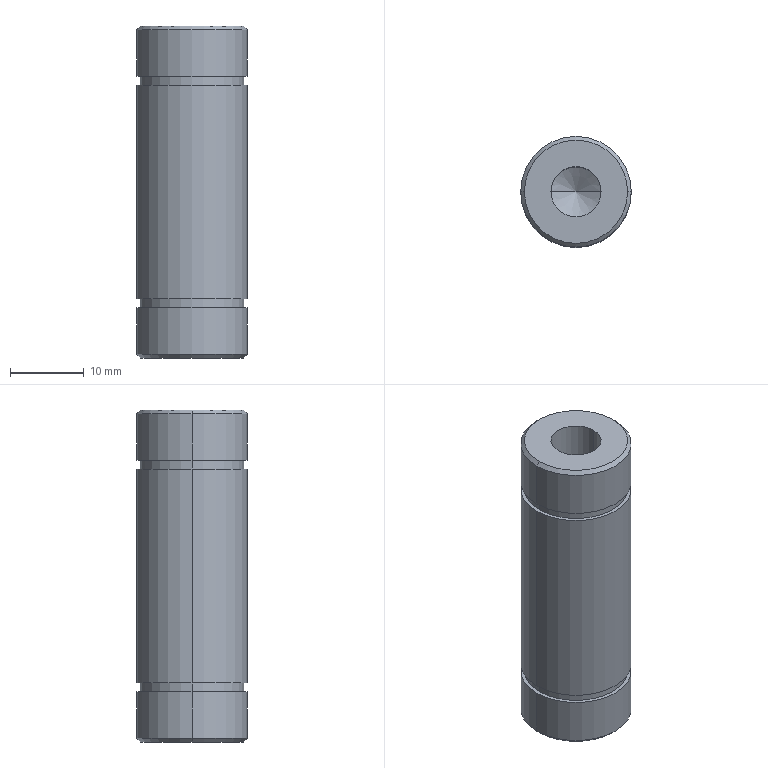Part | SolidWorks | features MirrorPattern 2, Chamfer 1, Extrusion 1, HoleWzd 1, RevCut 1 | 1 solid | 28 faces | box 15 x 15 x 45 mm | volume 6384 mm3 | cylinder 14 | cone 8 | plane 6 | commonest cylinder face diameters 15 x6 6.8 x4 14 x4
STEP:
#1=CARTESIAN_POINT('',(-7.5,0.,22.));
#2=VERTEX_POINT('',#1);
#3=CARTESIAN_POINT('',(7.5,0.,22.));
#4=VERTEX_POINT('',#3);
#5=CARTESIAN_POINT('',(0.,0.,22.));
#6=DIRECTION('',(0.,0.,-1.));
#7=DIRECTION('',(1.,0.,0.));
#8=AXIS2_PLACEMENT_3D('',#5,#6,#7);
#9=CIRCLE('',#8,7.5);
#10=EDGE_CURVE('',#2,#4,#9,.T.);
#11=ORIENTED_EDGE('',*,*,#10,.T.);
#12=CARTESIAN_POINT('',(7.5,0.,15.7));
#13=VERTEX_POINT('',#12);
#14=CARTESIAN_POINT('',(7.5,0.,22.5));
#15=DIRECTION('',(0.,0.,-1.));
#16=VECTOR('',#15,1000.);
#17=LINE('',#14,#16);
#18=EDGE_CURVE('',#4,#13,#17,.T.);
#19=ORIENTED_EDGE('',*,*,#18,.T.);
#20=CARTESIAN_POINT('',(-7.5,0.,15.7));
#21=VERTEX_POINT('',#20);
#22=CARTESIAN_POINT('',(0.,0.,15.7));
#23=DIRECTION('',(0.,0.,-1.));
#24=DIRECTION('',(-1.,0.,0.));
#25=AXIS2_PLACEMENT_3D('',#22,#23,#24);
#26=CIRCLE('',#25,7.5);
#27=EDGE_CURVE('',#21,#13,#26,.T.);
#28=ORIENTED_EDGE('',*,*,#27,.F.);
#29=CARTESIAN_POINT('',(-7.5,0.,22.5));
#30=DIRECTION('',(0.,0.,-1.));
#31=VECTOR('',#30,1000.);
#32=LINE('',#29,#31);
#33=EDGE_CURVE('',#2,#21,#32,.T.);
#34=ORIENTED_EDGE('',*,*,#33,.F.);
#35=EDGE_LOOP('',(#11,#19,#28,#34));
#36=FACE_OUTER_BOUND('',#35,.T.);
#37=CARTESIAN_POINT('',(0.,0.,22.5));
#38=DIRECTION('',(0.,0.,-1.));
#39=DIRECTION('',(-1.,0.,0.));
#40=AXIS2_PLACEMENT_3D('',#37,#38,#39);
#41=CYLINDRICAL_SURFACE('',#40,7.5);
#42=ADVANCED_FACE('',(#36),#41,.T.);
#43=CARTESIAN_POINT('',(7.,0.,22.5));
#44=VERTEX_POINT('',#43);
#45=CARTESIAN_POINT('',(-7.,0.,22.5));
#46=VERTEX_POINT('',#45);
#47=CARTESIAN_POINT('',(0.,0.,22.5));
#48=DIRECTION('',(0.,0.,1.));
#49=DIRECTION('',(1.,0.,0.));
#50=AXIS2_PLACEMENT_3D('',#47,#48,#49);
#51=CIRCLE('',#50,7.);
#52=EDGE_CURVE('',#44,#46,#51,.T.);
#53=ORIENTED_EDGE('',*,*,#52,.F.);
#54=CARTESIAN_POINT('',(7.,0.,22.5));
#55=DIRECTION('',(0.7071,0.,-0.7071));
#56=VECTOR('',#55,1000.);
#57=LINE('',#54,#56);
#58=EDGE_CURVE('',#44,#4,#57,.T.);
#59=ORIENTED_EDGE('',*,*,#58,.T.);
#60=ORIENTED_EDGE('',*,*,#10,.F.);
#61=CARTESIAN_POINT('',(-7.,0.,22.5));
#62=DIRECTION('',(-0.7071,0.,-0.7071));
#63=VECTOR('',#62,1000.);
#64=LINE('',#61,#63);
#65=EDGE_CURVE('',#46,#2,#64,.T.);
#66=ORIENTED_EDGE('',*,*,#65,.F.);
#67=EDGE_LOOP('',(#53,#59,#60,#66));
#68=FACE_OUTER_BOUND('',#67,.T.);
#69=CARTESIAN_POINT('',(0.,0.,22.5));
#70=DIRECTION('',(0.,0.,-1.));
#71=DIRECTION('',(-1.,0.,0.));
#72=AXIS2_PLACEMENT_3D('',#69,#70,#71);
#73=CONICAL_SURFACE('',#72,7.,0.7854);
#74=ADVANCED_FACE('',(#68),#73,.T.);
#75=CARTESIAN_POINT('',(-3.4,0.,2.5));
#76=VERTEX_POINT('',#75);
#77=CARTESIAN_POINT('',(3.4,0.,2.5));
#78=VERTEX_POINT('',#77);
#79=CARTESIAN_POINT('',(0.,0.,2.5));
#80=DIRECTION('',(0.,0.,1.));
#81=DIRECTION('',(1.,0.,0.));
#82=AXIS2_PLACEMENT_3D('',#79,#80,#81);
#83=CIRCLE('',#82,3.4);
#84=EDGE_CURVE('',#76,#78,#83,.T.);
#85=ORIENTED_EDGE('',*,*,#84,.F.);
#86=CARTESIAN_POINT('',(-3.4,0.,22.5));
#87=VERTEX_POINT('',#86);
#88=CARTESIAN_POINT('',(-3.4,0.,22.5));
#89=DIRECTION('',(0.,0.,1.));
#90=VECTOR('',#89,1000.);
#91=LINE('',#88,#90);
#92=EDGE_CURVE('',#76,#87,#91,.T.);
#93=ORIENTED_EDGE('',*,*,#92,.T.);
#94=CARTESIAN_POINT('',(3.4,0.,22.5));
#95=VERTEX_POINT('',#94);
#96=CARTESIAN_POINT('',(0.,0.,22.5));
#97=DIRECTION('',(0.,0.,1.));
#98=DIRECTION('',(1.,0.,0.));
#99=AXIS2_PLACEMENT_3D('',#96,#97,#98);
#100=CIRCLE('',#99,3.4);
#101=EDGE_CURVE('',#87,#95,#100,.T.);
#102=ORIENTED_EDGE('',*,*,#101,.T.);
#103=CARTESIAN_POINT('',(3.4,0.,22.5));
#104=DIRECTION('',(0.,0.,1.));
#105=VECTOR('',#104,1000.);
#106=LINE('',#103,#105);
#107=EDGE_CURVE('',#78,#95,#106,.T.);
#108=ORIENTED_EDGE('',*,*,#107,.F.);
#109=EDGE_LOOP('',(#85,#93,#102,#108));
#110=FACE_OUTER_BOUND('',#109,.T.);
#111=CARTESIAN_POINT('',(0.,0.,22.5));
#112=DIRECTION('',(0.,0.,1.));
#113=DIRECTION('',(1.,0.,0.));
#114=AXIS2_PLACEMENT_3D('',#111,#112,#113);
#115=CYLINDRICAL_SURFACE('',#114,3.4);
#116=ADVANCED_FACE('',(#110),#115,.F.);
#117=CARTESIAN_POINT('',(0.,0.,0.4571));
#118=VERTEX_POINT('',#117);
#119=CARTESIAN_POINT('',(3.4,0.,2.5));
#120=DIRECTION('',(0.8572,0.,0.515));
#121=VECTOR('',#120,1000.);
#122=LINE('',#119,#121);
#123=EDGE_CURVE('',#118,#78,#122,.T.);
#124=ORIENTED_EDGE('',*,*,#123,.F.);
#125=CARTESIAN_POINT('',(-3.4,0.,2.5));
#126=DIRECTION('',(-0.8572,0.,0.515));
#127=VECTOR('',#126,1000.);
#128=LINE('',#125,#127);
#129=EDGE_CURVE('',#118,#76,#128,.T.);
#130=ORIENTED_EDGE('',*,*,#129,.T.);
#131=ORIENTED_EDGE('',*,*,#84,.T.);
#132=EDGE_LOOP('',(#124,#130,#131));
#133=FACE_OUTER_BOUND('',#132,.T.);
#134=CARTESIAN_POINT('',(0.,0.,2.5));
#135=DIRECTION('',(0.,0.,1.));
#136=DIRECTION('',(1.,0.,0.));
#137=AXIS2_PLACEMENT_3D('',#134,#135,#136);
#138=CONICAL_SURFACE('',#137,3.4,1.03);
#139=ADVANCED_FACE('',(#133),#138,.F.);
#140=CARTESIAN_POINT('',(7.,0.,14.5));
#141=VERTEX_POINT('',#140);
#142=CARTESIAN_POINT('',(-7.,0.,14.5));
#143=VERTEX_POINT('',#142);
#144=CARTESIAN_POINT('',(0.,0.,14.5));
#145=DIRECTION('',(0.,0.,-1.));
#146=DIRECTION('',(-1.,0.,0.));
#147=AXIS2_PLACEMENT_3D('',#144,#145,#146);
#148=CIRCLE('',#147,7.);
#149=EDGE_CURVE('',#141,#143,#148,.T.);
#150=ORIENTED_EDGE('',*,*,#149,.F.);
#151=CARTESIAN_POINT('',(7.,0.,15.7));
#152=VERTEX_POINT('',#151);
#153=CARTESIAN_POINT('',(7.,0.,24.689));
#154=DIRECTION('',(0.,0.,1.));
#155=VECTOR('',#154,1000.);
#156=LINE('',#153,#155);
#157=EDGE_CURVE('',#141,#152,#156,.T.);
#158=ORIENTED_EDGE('',*,*,#157,.T.);
#159=CARTESIAN_POINT('',(-7.,0.,15.7));
#160=VERTEX_POINT('',#159);
#161=CARTESIAN_POINT('',(0.,0.,15.7));
#162=DIRECTION('',(0.,0.,-1.));
#163=DIRECTION('',(-1.,0.,0.));
#164=AXIS2_PLACEMENT_3D('',#161,#162,#163);
#165=CIRCLE('',#164,7.);
#166=EDGE_CURVE('',#152,#160,#165,.T.);
#167=ORIENTED_EDGE('',*,*,#166,.T.);
#168=CARTESIAN_POINT('',(-7.,0.,24.689));
#169=DIRECTION('',(0.,0.,1.));
#170=VECTOR('',#169,1000.);
#171=LINE('',#168,#170);
#172=EDGE_CURVE('',#143,#160,#171,.T.);
#173=ORIENTED_EDGE('',*,*,#172,.F.);
#174=EDGE_LOOP('',(#150,#158,#167,#173));
#175=FACE_OUTER_BOUND('',#174,.T.);
#176=CARTESIAN_POINT('',(0.,0.,24.689));
#177=DIRECTION('',(0.,0.,1.));
#178=DIRECTION('',(-1.,0.,0.));
#179=AXIS2_PLACEMENT_3D('',#176,#177,#178);
#180=CYLINDRICAL_SURFACE('',#179,7.);
#181=ADVANCED_FACE('',(#175),#180,.T.);
#182=CARTESIAN_POINT('',(-7.5,0.,-15.7));
#183=VERTEX_POINT('',#182);
#184=CARTESIAN_POINT('',(7.5,0.,-15.7));
#185=VERTEX_POINT('',#184);
#186=CARTESIAN_POINT('',(0.,0.,-15.7));
#187=DIRECTION('',(0.,0.,-1.));
#188=DIRECTION('',(-1.,0.,0.));
#189=AXIS2_PLACEMENT_3D('',#186,#187,#188);
#190=CIRCLE('',#189,7.5);
#191=EDGE_CURVE('',#183,#185,#190,.T.);
#192=ORIENTED_EDGE('',*,*,#191,.T.);
#193=CARTESIAN_POINT('',(7.5,0.,-22.));
#194=VERTEX_POINT('',#193);
#195=CARTESIAN_POINT('',(7.5,0.,22.5));
#196=DIRECTION('',(0.,0.,-1.));
#197=VECTOR('',#196,1000.);
#198=LINE('',#195,#197);
#199=EDGE_CURVE('',#185,#194,#198,.T.);
#200=ORIENTED_EDGE('',*,*,#199,.T.);
#201=CARTESIAN_POINT('',(-7.5,0.,-22.));
#202=VERTEX_POINT('',#201);
#203=CARTESIAN_POINT('',(0.,0.,-22.));
#204=DIRECTION('',(0.,0.,1.));
#205=DIRECTION('',(1.,0.,0.));
#206=AXIS2_PLACEMENT_3D('',#203,#204,#205);
#207=CIRCLE('',#206,7.5);
#208=EDGE_CURVE('',#194,#202,#207,.T.);
#209=ORIENTED_EDGE('',*,*,#208,.T.);
#210=CARTESIAN_POINT('',(-7.5,0.,22.5));
#211=DIRECTION('',(0.,0.,-1.));
#212=VECTOR('',#211,1000.);
#213=LINE('',#210,#212);
#214=EDGE_CURVE('',#183,#202,#213,.T.);
#215=ORIENTED_EDGE('',*,*,#214,.F.);
#216=EDGE_LOOP('',(#192,#200,#209,#215));
#217=FACE_OUTER_BOUND('',#216,.T.);
#218=CARTESIAN_POINT('',(0.,0.,22.5));
#219=DIRECTION('',(0.,0.,-1.));
#220=DIRECTION('',(-1.,0.,0.));
#221=AXIS2_PLACEMENT_3D('',#218,#219,#220);
#222=CYLINDRICAL_SURFACE('',#221,7.5);
#223=ADVANCED_FACE('',(#217),#222,.T.);
#224=CARTESIAN_POINT('',(-7.,0.,-22.5));
#225=VERTEX_POINT('',#224);
#226=CARTESIAN_POINT('',(7.,0.,-22.5));
#227=VERTEX_POINT('',#226);
#228=CARTESIAN_POINT('',(0.,0.,-22.5));
#229=DIRECTION('',(0.,0.,-1.));
#230=DIRECTION('',(1.,0.,0.));
#231=AXIS2_PLACEMENT_3D('',#228,#229,#230);
#232=CIRCLE('',#231,7.);
#233=EDGE_CURVE('',#225,#227,#232,.T.);
#234=ORIENTED_EDGE('',*,*,#233,.F.);
#235=CARTESIAN_POINT('',(-7.5,0.,-22.));
#236=DIRECTION('',(-0.7071,0.,0.7071));
#237=VECTOR('',#236,1000.);
#238=LINE('',#235,#237);
#239=EDGE_CURVE('',#225,#202,#238,.T.);
#240=ORIENTED_EDGE('',*,*,#239,.T.);
#241=ORIENTED_EDGE('',*,*,#208,.F.);
#242=CARTESIAN_POINT('',(7.5,0.,-22.));
#243=DIRECTION('',(0.7071,0.,0.7071));
#244=VECTOR('',#243,1000.);
#245=LINE('',#242,#244);
#246=EDGE_CURVE('',#227,#194,#245,.T.);
#247=ORIENTED_EDGE('',*,*,#246,.F.);
#248=EDGE_LOOP('',(#234,#240,#241,#247));
#249=FACE_OUTER_BOUND('',#248,.T.);
#250=CARTESIAN_POINT('',(0.,0.,-22.));
#251=DIRECTION('',(0.,0.,1.));
#252=DIRECTION('',(1.,0.,0.));
#253=AXIS2_PLACEMENT_3D('',#250,#251,#252);
#254=CONICAL_SURFACE('',#253,7.5,0.7854);
#255=ADVANCED_FACE('',(#249),#254,.T.);
#256=CARTESIAN_POINT('',(3.4,0.,-2.5));
#257=VERTEX_POINT('',#256);
#258=CARTESIAN_POINT('',(-3.4,0.,-2.5));
#259=VERTEX_POINT('',#258);
#260=CARTESIAN_POINT('',(0.,0.,-2.5));
#261=DIRECTION('',(0.,0.,-1.));
#262=DIRECTION('',(-1.,0.,0.));
#263=AXIS2_PLACEMENT_3D('',#260,#261,#262);
#264=CIRCLE('',#263,3.4);
#265=EDGE_CURVE('',#257,#259,#264,.T.);
#266=ORIENTED_EDGE('',*,*,#265,.F.);
#267=CARTESIAN_POINT('',(3.4,0.,-22.5));
#268=VERTEX_POINT('',#267);
#269=CARTESIAN_POINT('',(3.4,0.,-22.5));
#270=DIRECTION('',(0.,0.,-1.));
#271=VECTOR('',#270,1000.);
#272=LINE('',#269,#271);
#273=EDGE_CURVE('',#257,#268,#272,.T.);
#274=ORIENTED_EDGE('',*,*,#273,.T.);
#275=CARTESIAN_POINT('',(-3.4,0.,-22.5));
#276=VERTEX_POINT('',#275);
#277=CARTESIAN_POINT('',(0.,0.,-22.5));
#278=DIRECTION('',(0.,0.,-1.));
#279=DIRECTION('',(-1.,0.,0.));
#280=AXIS2_PLACEMENT_3D('',#277,#278,#279);
#281=CIRCLE('',#280,3.4);
#282=EDGE_CURVE('',#268,#276,#281,.T.);
#283=ORIENTED_EDGE('',*,*,#282,.T.);
#284=CARTESIAN_POINT('',(-3.4,0.,-22.5));
#285=DIRECTION('',(0.,0.,-1.));
#286=VECTOR('',#285,1000.);
#287=LINE('',#284,#286);
#288=EDGE_CURVE('',#259,#276,#287,.T.);
#289=ORIENTED_EDGE('',*,*,#288,.F.);
#290=EDGE_LOOP('',(#266,#274,#283,#289));
#291=FACE_OUTER_BOUND('',#290,.T.);
#292=CARTESIAN_POINT('',(0.,0.,-22.5));
#293=DIRECTION('',(0.,0.,-1.));
#294=DIRECTION('',(-1.,0.,0.));
#295=AXIS2_PLACEMENT_3D('',#292,#293,#294);
#296=CYLINDRICAL_SURFACE('',#295,3.4);
#297=ADVANCED_FACE('',(#291),#296,.F.);
#298=CARTESIAN_POINT('',(0.,0.,-0.4571));
#299=VERTEX_POINT('',#298);
#300=CARTESIAN_POINT('',(-3.4,0.,-2.5));
#301=DIRECTION('',(-0.8572,0.,-0.515));
#302=VECTOR('',#301,1000.);
#303=LINE('',#300,#302);
#304=EDGE_CURVE('',#299,#259,#303,.T.);
#305=ORIENTED_EDGE('',*,*,#304,.F.);
#306=CARTESIAN_POINT('',(3.4,0.,-2.5));
#307=DIRECTION('',(0.8572,0.,-0.515));
#308=VECTOR('',#307,1000.);
#309=LINE('',#306,#308);
#310=EDGE_CURVE('',#299,#257,#309,.T.);
#311=ORIENTED_EDGE('',*,*,#310,.T.);
#312=ORIENTED_EDGE('',*,*,#265,.T.);
#313=EDGE_LOOP('',(#305,#311,#312));
#314=FACE_OUTER_BOUND('',#313,.T.);
#315=CARTESIAN_POINT('',(0.,0.,-2.5));
#316=DIRECTION('',(0.,0.,-1.));
#317=DIRECTION('',(-1.,0.,0.));
#318=AXIS2_PLACEMENT_3D('',#315,#316,#317);
#319=CONICAL_SURFACE('',#318,3.4,1.03);
#320=ADVANCED_FACE('',(#314),#319,.F.);
#321=CARTESIAN_POINT('',(-7.,0.,-14.5));
#322=VERTEX_POINT('',#321);
#323=CARTESIAN_POINT('',(7.,0.,-14.5));
#324=VERTEX_POINT('',#323);
#325=CARTESIAN_POINT('',(0.,0.,-14.5));
#326=DIRECTION('',(0.,0.,-1.));
#327=DIRECTION('',(-1.,0.,0.));
#328=AXIS2_PLACEMENT_3D('',#325,#326,#327);
#329=CIRCLE('',#328,7.);
#330=EDGE_CURVE('',#322,#324,#329,.T.);
#331=ORIENTED_EDGE('',*,*,#330,.T.);
#332=CARTESIAN_POINT('',(7.,0.,-15.7));
#333=VERTEX_POINT('',#332);
#334=CARTESIAN_POINT('',(7.,0.,-24.689));
#335=DIRECTION('',(0.,0.,-1.));
#336=VECTOR('',#335,1000.);
#337=LINE('',#334,#336);
#338=EDGE_CURVE('',#324,#333,#337,.T.);
#339=ORIENTED_EDGE('',*,*,#338,.T.);
#340=CARTESIAN_POINT('',(-7.,0.,-15.7));
#341=VERTEX_POINT('',#340);
#342=CARTESIAN_POINT('',(0.,0.,-15.7));
#343=DIRECTION('',(0.,0.,-1.));
#344=DIRECTION('',(-1.,0.,0.));
#345=AXIS2_PLACEMENT_3D('',#342,#343,#344);
#346=CIRCLE('',#345,7.);
#347=EDGE_CURVE('',#341,#333,#346,.T.);
#348=ORIENTED_EDGE('',*,*,#347,.F.);
#349=CARTESIAN_POINT('',(-7.,0.,-24.689));
#350=DIRECTION('',(0.,0.,-1.));
#351=VECTOR('',#350,1000.);
#352=LINE('',#349,#351);
#353=EDGE_CURVE('',#322,#341,#352,.T.);
#354=ORIENTED_EDGE('',*,*,#353,.F.);
#355=EDGE_LOOP('',(#331,#339,#348,#354));
#356=FACE_OUTER_BOUND('',#355,.T.);
#357=CARTESIAN_POINT('',(0.,0.,-24.689));
#358=DIRECTION('',(0.,0.,-1.));
#359=DIRECTION('',(-1.,0.,0.));
#360=AXIS2_PLACEMENT_3D('',#357,#358,#359);
#361=CYLINDRICAL_SURFACE('',#360,7.);
#362=ADVANCED_FACE('',(#356),#361,.T.);
#363=CARTESIAN_POINT('',(-7.5,0.,14.5));
#364=VERTEX_POINT('',#363);
#365=CARTESIAN_POINT('',(7.5,0.,14.5));
#366=VERTEX_POINT('',#365);
#367=CARTESIAN_POINT('',(0.,0.,14.5));
#368=DIRECTION('',(0.,0.,-1.));
#369=DIRECTION('',(-1.,0.,0.));
#370=AXIS2_PLACEMENT_3D('',#367,#368,#369);
#371=CIRCLE('',#370,7.5);
#372=EDGE_CURVE('',#364,#366,#371,.T.);
#373=ORIENTED_EDGE('',*,*,#372,.T.);
#374=CARTESIAN_POINT('',(7.5,0.,-14.5));
#375=VERTEX_POINT('',#374);
#376=CARTESIAN_POINT('',(7.5,0.,22.5));
#377=DIRECTION('',(0.,0.,-1.));
#378=VECTOR('',#377,1000.);
#379=LINE('',#376,#378);
#380=EDGE_CURVE('',#366,#375,#379,.T.);
#381=ORIENTED_EDGE('',*,*,#380,.T.);
#382=CARTESIAN_POINT('',(-7.5,0.,-14.5));
#383=VERTEX_POINT('',#382);
#384=CARTESIAN_POINT('',(0.,0.,-14.5));
#385=DIRECTION('',(0.,0.,-1.));
#386=DIRECTION('',(-1.,0.,0.));
#387=AXIS2_PLACEMENT_3D('',#384,#385,#386);
#388=CIRCLE('',#387,7.5);
#389=EDGE_CURVE('',#383,#375,#388,.T.);
#390=ORIENTED_EDGE('',*,*,#389,.F.);
#391=CARTESIAN_POINT('',(-7.5,0.,22.5));
#392=DIRECTION('',(0.,0.,-1.));
#393=VECTOR('',#392,1000.);
#394=LINE('',#391,#393);
#395=EDGE_CURVE('',#364,#383,#394,.T.);
#396=ORIENTED_EDGE('',*,*,#395,.F.);
#397=EDGE_LOOP('',(#373,#381,#390,#396));
#398=FACE_OUTER_BOUND('',#397,.T.);
#399=CARTESIAN_POINT('',(0.,0.,22.5));
#400=DIRECTION('',(0.,0.,-1.));
#401=DIRECTION('',(-1.,0.,0.));
#402=AXIS2_PLACEMENT_3D('',#399,#400,#401);
#403=CYLINDRICAL_SURFACE('',#402,7.5);
#404=ADVANCED_FACE('',(#398),#403,.T.);
#405=ORIENTED_EDGE('',*,*,#380,.F.);
#406=CARTESIAN_POINT('',(0.,0.,14.5));
#407=DIRECTION('',(0.,0.,-1.));
#408=DIRECTION('',(-1.,0.,0.));
#409=AXIS2_PLACEMENT_3D('',#406,#407,#408);
#410=CIRCLE('',#409,7.5);
#411=EDGE_CURVE('',#366,#364,#410,.T.);
#412=ORIENTED_EDGE('',*,*,#411,.T.);
#413=ORIENTED_EDGE('',*,*,#395,.T.);
#414=CARTESIAN_POINT('',(0.,0.,-14.5));
#415=DIRECTION('',(0.,0.,-1.));
#416=DIRECTION('',(-1.,0.,0.));
#417=AXIS2_PLACEMENT_3D('',#414,#415,#416);
#418=CIRCLE('',#417,7.5);
#419=EDGE_CURVE('',#375,#383,#418,.T.);
#420=ORIENTED_EDGE('',*,*,#419,.F.);
#421=EDGE_LOOP('',(#405,#412,#413,#420));
#422=FACE_OUTER_BOUND('',#421,.T.);
#423=CARTESIAN_POINT('',(0.,0.,22.5));
#424=DIRECTION('',(0.,0.,-1.));
#425=DIRECTION('',(-1.,0.,0.));
#426=AXIS2_PLACEMENT_3D('',#423,#424,#425);
#427=CYLINDRICAL_SURFACE('',#426,7.5);
#428=ADVANCED_FACE('',(#422),#427,.T.);
#429=ORIENTED_EDGE('',*,*,#389,.T.);
#430=ORIENTED_EDGE('',*,*,#419,.T.);
#431=EDGE_LOOP('',(#429,#430));
#432=FACE_OUTER_BOUND('',#431,.T.);
#433=ORIENTED_EDGE('',*,*,#330,.F.);
#434=CARTESIAN_POINT('',(0.,0.,-14.5));
#435=DIRECTION('',(0.,0.,-1.));
#436=DIRECTION('',(-1.,0.,0.));
#437=AXIS2_PLACEMENT_3D('',#434,#435,#436);
#438=CIRCLE('',#437,7.);
#439=EDGE_CURVE('',#324,#322,#438,.T.);
#440=ORIENTED_EDGE('',*,*,#439,.F.);
#441=EDGE_LOOP('',(#433,#440));
#442=FACE_BOUND('',#441,.T.);
#443=CARTESIAN_POINT('',(7.5,0.,-14.5));
#444=DIRECTION('',(0.,0.,-1.));
#445=DIRECTION('',(-1.,0.,0.));
#446=AXIS2_PLACEMENT_3D('',#443,#444,#445);
#447=PLANE('',#446);
#448=ADVANCED_FACE('',(#432,#442),#447,.T.);
#449=ORIENTED_EDGE('',*,*,#338,.F.);
#450=ORIENTED_EDGE('',*,*,#439,.T.);
#451=ORIENTED_EDGE('',*,*,#353,.T.);
#452=CARTESIAN_POINT('',(0.,0.,-15.7));
#453=DIRECTION('',(0.,0.,-1.));
#454=DIRECTION('',(-1.,0.,0.));
#455=AXIS2_PLACEMENT_3D('',#452,#453,#454);
#456=CIRCLE('',#455,7.);
#457=EDGE_CURVE('',#333,#341,#456,.T.);
#458=ORIENTED_EDGE('',*,*,#457,.F.);
#459=EDGE_LOOP('',(#449,#450,#451,#458));
#460=FACE_OUTER_BOUND('',#459,.T.);
#461=CARTESIAN_POINT('',(0.,0.,-24.689));
#462=DIRECTION('',(0.,0.,-1.));
#463=DIRECTION('',(-1.,0.,0.));
#464=AXIS2_PLACEMENT_3D('',#461,#462,#463);
#465=CYLINDRICAL_SURFACE('',#464,7.);
#466=ADVANCED_FACE('',(#460),#465,.T.);
#467=ORIENTED_EDGE('',*,*,#347,.T.);
#468=ORIENTED_EDGE('',*,*,#457,.T.);
#469=EDGE_LOOP('',(#467,#468));
#470=FACE_BOUND('',#469,.T.);
#471=ORIENTED_EDGE('',*,*,#191,.F.);
#472=CARTESIAN_POINT('',(0.,0.,-15.7));
#473=DIRECTION('',(0.,0.,-1.));
#474=DIRECTION('',(-1.,0.,0.));
#475=AXIS2_PLACEMENT_3D('',#472,#473,#474);
#476=CIRCLE('',#475,7.5);
#477=EDGE_CURVE('',#185,#183,#476,.T.);
#478=ORIENTED_EDGE('',*,*,#477,.F.);
#479=EDGE_LOOP('',(#471,#478));
#480=FACE_OUTER_BOUND('',#479,.T.);
#481=CARTESIAN_POINT('',(7.5,0.,-15.7));
#482=DIRECTION('',(0.,0.,1.));
#483=DIRECTION('',(1.,0.,0.));
#484=AXIS2_PLACEMENT_3D('',#481,#482,#483);
#485=PLANE('',#484);
#486=ADVANCED_FACE('',(#470,#480),#485,.T.);
#487=ORIENTED_EDGE('',*,*,#310,.F.);
#488=ORIENTED_EDGE('',*,*,#304,.T.);
#489=CARTESIAN_POINT('',(0.,0.,-2.5));
#490=DIRECTION('',(0.,0.,-1.));
#491=DIRECTION('',(-1.,0.,0.));
#492=AXIS2_PLACEMENT_3D('',#489,#490,#491);
#493=CIRCLE('',#492,3.4);
#494=EDGE_CURVE('',#259,#257,#493,.T.);
#495=ORIENTED_EDGE('',*,*,#494,.T.);
#496=EDGE_LOOP('',(#487,#488,#495));
#497=FACE_OUTER_BOUND('',#496,.T.);
#498=CARTESIAN_POINT('',(0.,0.,-2.5));
#499=DIRECTION('',(0.,0.,-1.));
#500=DIRECTION('',(-1.,0.,0.));
#501=AXIS2_PLACEMENT_3D('',#498,#499,#500);
#502=CONICAL_SURFACE('',#501,3.4,1.03);
#503=ADVANCED_FACE('',(#497),#502,.F.);
#504=ORIENTED_EDGE('',*,*,#273,.F.);
#505=ORIENTED_EDGE('',*,*,#494,.F.);
#506=ORIENTED_EDGE('',*,*,#288,.T.);
#507=CARTESIAN_POINT('',(0.,0.,-22.5));
#508=DIRECTION('',(0.,0.,-1.));
#509=DIRECTION('',(-1.,0.,0.));
#510=AXIS2_PLACEMENT_3D('',#507,#508,#509);
#511=CIRCLE('',#510,3.4);
#512=EDGE_CURVE('',#276,#268,#511,.T.);
#513=ORIENTED_EDGE('',*,*,#512,.T.);
#514=EDGE_LOOP('',(#504,#505,#506,#513));
#515=FACE_OUTER_BOUND('',#514,.T.);
#516=CARTESIAN_POINT('',(0.,0.,-22.5));
#517=DIRECTION('',(0.,0.,-1.));
#518=DIRECTION('',(-1.,0.,0.));
#519=AXIS2_PLACEMENT_3D('',#516,#517,#518);
#520=CYLINDRICAL_SURFACE('',#519,3.4);
#521=ADVANCED_FACE('',(#515),#520,.F.);
#522=ORIENTED_EDGE('',*,*,#512,.F.);
#523=ORIENTED_EDGE('',*,*,#282,.F.);
#524=EDGE_LOOP('',(#522,#523));
#525=FACE_BOUND('',#524,.T.);
#526=CARTESIAN_POINT('',(0.,0.,-22.5));
#527=DIRECTION('',(0.,0.,-1.));
#528=DIRECTION('',(1.,0.,0.));
#529=AXIS2_PLACEMENT_3D('',#526,#527,#528);
#530=CIRCLE('',#529,7.);
#531=EDGE_CURVE('',#227,#225,#530,.T.);
#532=ORIENTED_EDGE('',*,*,#531,.T.);
#533=ORIENTED_EDGE('',*,*,#233,.T.);
#534=EDGE_LOOP('',(#532,#533));
#535=FACE_OUTER_BOUND('',#534,.T.);
#536=CARTESIAN_POINT('',(0.,0.,-22.5));
#537=DIRECTION('',(0.,0.,1.));
#538=DIRECTION('',(1.,0.,0.));
#539=AXIS2_PLACEMENT_3D('',#536,#537,#538);
#540=PLANE('',#539);
#541=ADVANCED_FACE('',(#525,#535),#540,.F.);
#542=ORIENTED_EDGE('',*,*,#239,.F.);
#543=ORIENTED_EDGE('',*,*,#531,.F.);
#544=ORIENTED_EDGE('',*,*,#246,.T.);
#545=CARTESIAN_POINT('',(0.,0.,-22.));
#546=DIRECTION('',(0.,0.,1.));
#547=DIRECTION('',(1.,0.,0.));
#548=AXIS2_PLACEMENT_3D('',#545,#546,#547);
#549=CIRCLE('',#548,7.5);
#550=EDGE_CURVE('',#202,#194,#549,.T.);
#551=ORIENTED_EDGE('',*,*,#550,.F.);
#552=EDGE_LOOP('',(#542,#543,#544,#551));
#553=FACE_OUTER_BOUND('',#552,.T.);
#554=CARTESIAN_POINT('',(0.,0.,-22.));
#555=DIRECTION('',(0.,0.,1.));
#556=DIRECTION('',(1.,0.,0.));
#557=AXIS2_PLACEMENT_3D('',#554,#555,#556);
#558=CONICAL_SURFACE('',#557,7.5,0.7854);
#559=ADVANCED_FACE('',(#553),#558,.T.);
#560=ORIENTED_EDGE('',*,*,#199,.F.);
#561=ORIENTED_EDGE('',*,*,#477,.T.);
#562=ORIENTED_EDGE('',*,*,#214,.T.);
#563=ORIENTED_EDGE('',*,*,#550,.T.);
#564=EDGE_LOOP('',(#560,#561,#562,#563));
#565=FACE_OUTER_BOUND('',#564,.T.);
#566=CARTESIAN_POINT('',(0.,0.,22.5));
#567=DIRECTION('',(0.,0.,-1.));
#568=DIRECTION('',(-1.,0.,0.));
#569=AXIS2_PLACEMENT_3D('',#566,#567,#568);
#570=CYLINDRICAL_SURFACE('',#569,7.5);
#571=ADVANCED_FACE('',(#565),#570,.T.);
#572=ORIENTED_EDGE('',*,*,#372,.F.);
#573=ORIENTED_EDGE('',*,*,#411,.F.);
#574=EDGE_LOOP('',(#572,#573));
#575=FACE_OUTER_BOUND('',#574,.T.);
#576=CARTESIAN_POINT('',(0.,0.,14.5));
#577=DIRECTION('',(0.,0.,-1.));
#578=DIRECTION('',(-1.,0.,0.));
#579=AXIS2_PLACEMENT_3D('',#576,#577,#578);
#580=CIRCLE('',#579,7.);
#581=EDGE_CURVE('',#143,#141,#580,.T.);
#582=ORIENTED_EDGE('',*,*,#581,.T.);
#583=ORIENTED_EDGE('',*,*,#149,.T.);
#584=EDGE_LOOP('',(#582,#583));
#585=FACE_BOUND('',#584,.T.);
#586=CARTESIAN_POINT('',(7.5,0.,14.5));
#587=DIRECTION('',(0.,0.,1.));
#588=DIRECTION('',(-1.,0.,0.));
#589=AXIS2_PLACEMENT_3D('',#586,#587,#588);
#590=PLANE('',#589);
#591=ADVANCED_FACE('',(#575,#585),#590,.T.);
#592=ORIENTED_EDGE('',*,*,#157,.F.);
#593=ORIENTED_EDGE('',*,*,#581,.F.);
#594=ORIENTED_EDGE('',*,*,#172,.T.);
#595=CARTESIAN_POINT('',(0.,0.,15.7));
#596=DIRECTION('',(0.,0.,-1.));
#597=DIRECTION('',(-1.,0.,0.));
#598=AXIS2_PLACEMENT_3D('',#595,#596,#597);
#599=CIRCLE('',#598,7.);
#600=EDGE_CURVE('',#160,#152,#599,.T.);
#601=ORIENTED_EDGE('',*,*,#600,.T.);
#602=EDGE_LOOP('',(#592,#593,#594,#601));
#603=FACE_OUTER_BOUND('',#602,.T.);
#604=CARTESIAN_POINT('',(0.,0.,24.689));
#605=DIRECTION('',(0.,0.,1.));
#606=DIRECTION('',(-1.,0.,0.));
#607=AXIS2_PLACEMENT_3D('',#604,#605,#606);
#608=CYLINDRICAL_SURFACE('',#607,7.);
#609=ADVANCED_FACE('',(#603),#608,.T.);
#610=ORIENTED_EDGE('',*,*,#600,.F.);
#611=ORIENTED_EDGE('',*,*,#166,.F.);
#612=EDGE_LOOP('',(#610,#611));
#613=FACE_BOUND('',#612,.T.);
#614=ORIENTED_EDGE('',*,*,#27,.T.);
#615=CARTESIAN_POINT('',(0.,0.,15.7));
#616=DIRECTION('',(0.,0.,-1.));
#617=DIRECTION('',(-1.,0.,0.));
#618=AXIS2_PLACEMENT_3D('',#615,#616,#617);
#619=CIRCLE('',#618,7.5);
#620=EDGE_CURVE('',#13,#21,#619,.T.);
#621=ORIENTED_EDGE('',*,*,#620,.T.);
#622=EDGE_LOOP('',(#614,#621));
#623=FACE_OUTER_BOUND('',#622,.T.);
#624=CARTESIAN_POINT('',(7.5,0.,15.7));
#625=DIRECTION('',(0.,0.,-1.));
#626=DIRECTION('',(1.,0.,0.));
#627=AXIS2_PLACEMENT_3D('',#624,#625,#626);
#628=PLANE('',#627);
#629=ADVANCED_FACE('',(#613,#623),#628,.T.);
#630=ORIENTED_EDGE('',*,*,#129,.F.);
#631=ORIENTED_EDGE('',*,*,#123,.T.);
#632=CARTESIAN_POINT('',(0.,0.,2.5));
#633=DIRECTION('',(0.,0.,1.));
#634=DIRECTION('',(1.,0.,0.));
#635=AXIS2_PLACEMENT_3D('',#632,#633,#634);
#636=CIRCLE('',#635,3.4);
#637=EDGE_CURVE('',#78,#76,#636,.T.);
#638=ORIENTED_EDGE('',*,*,#637,.T.);
#639=EDGE_LOOP('',(#630,#631,#638));
#640=FACE_OUTER_BOUND('',#639,.T.);
#641=CARTESIAN_POINT('',(0.,0.,2.5));
#642=DIRECTION('',(0.,0.,1.));
#643=DIRECTION('',(1.,0.,0.));
#644=AXIS2_PLACEMENT_3D('',#641,#642,#643);
#645=CONICAL_SURFACE('',#644,3.4,1.03);
#646=ADVANCED_FACE('',(#640),#645,.F.);
#647=ORIENTED_EDGE('',*,*,#92,.F.);
#648=ORIENTED_EDGE('',*,*,#637,.F.);
#649=ORIENTED_EDGE('',*,*,#107,.T.);
#650=CARTESIAN_POINT('',(0.,0.,22.5));
#651=DIRECTION('',(0.,0.,1.));
#652=DIRECTION('',(1.,0.,0.));
#653=AXIS2_PLACEMENT_3D('',#650,#651,#652);
#654=CIRCLE('',#653,3.4);
#655=EDGE_CURVE('',#95,#87,#654,.T.);
#656=ORIENTED_EDGE('',*,*,#655,.T.);
#657=EDGE_LOOP('',(#647,#648,#649,#656));
#658=FACE_OUTER_BOUND('',#657,.T.);
#659=CARTESIAN_POINT('',(0.,0.,22.5));
#660=DIRECTION('',(0.,0.,1.));
#661=DIRECTION('',(1.,0.,0.));
#662=AXIS2_PLACEMENT_3D('',#659,#660,#661);
#663=CYLINDRICAL_SURFACE('',#662,3.4);
#664=ADVANCED_FACE('',(#658),#663,.F.);
#665=CARTESIAN_POINT('',(0.,0.,22.5));
#666=DIRECTION('',(0.,0.,1.));
#667=DIRECTION('',(1.,0.,0.));
#668=AXIS2_PLACEMENT_3D('',#665,#666,#667);
#669=CIRCLE('',#668,7.);
#670=EDGE_CURVE('',#46,#44,#669,.T.);
#671=ORIENTED_EDGE('',*,*,#670,.T.);
#672=ORIENTED_EDGE('',*,*,#52,.T.);
#673=EDGE_LOOP('',(#671,#672));
#674=FACE_OUTER_BOUND('',#673,.T.);
#675=ORIENTED_EDGE('',*,*,#655,.F.);
#676=ORIENTED_EDGE('',*,*,#101,.F.);
#677=EDGE_LOOP('',(#675,#676));
#678=FACE_BOUND('',#677,.T.);
#679=CARTESIAN_POINT('',(0.,0.,22.5));
#680=DIRECTION('',(0.,0.,1.));
#681=DIRECTION('',(1.,0.,0.));
#682=AXIS2_PLACEMENT_3D('',#679,#680,#681);
#683=PLANE('',#682);
#684=ADVANCED_FACE('',(#674,#678),#683,.T.);
#685=ORIENTED_EDGE('',*,*,#58,.F.);
#686=ORIENTED_EDGE('',*,*,#670,.F.);
#687=ORIENTED_EDGE('',*,*,#65,.T.);
#688=CARTESIAN_POINT('',(0.,0.,22.));
#689=DIRECTION('',(0.,0.,-1.));
#690=DIRECTION('',(1.,0.,0.));
#691=AXIS2_PLACEMENT_3D('',#688,#689,#690);
#692=CIRCLE('',#691,7.5);
#693=EDGE_CURVE('',#4,#2,#692,.T.);
#694=ORIENTED_EDGE('',*,*,#693,.F.);
#695=EDGE_LOOP('',(#685,#686,#687,#694));
#696=FACE_OUTER_BOUND('',#695,.T.);
#697=CARTESIAN_POINT('',(0.,0.,22.5));
#698=DIRECTION('',(0.,0.,-1.));
#699=DIRECTION('',(-1.,0.,0.));
#700=AXIS2_PLACEMENT_3D('',#697,#698,#699);
#701=CONICAL_SURFACE('',#700,7.,0.7854);
#702=ADVANCED_FACE('',(#696),#701,.T.);
#703=ORIENTED_EDGE('',*,*,#18,.F.);
#704=ORIENTED_EDGE('',*,*,#693,.T.);
#705=ORIENTED_EDGE('',*,*,#33,.T.);
#706=ORIENTED_EDGE('',*,*,#620,.F.);
#707=EDGE_LOOP('',(#703,#704,#705,#706));
#708=FACE_OUTER_BOUND('',#707,.T.);
#709=CARTESIAN_POINT('',(0.,0.,22.5));
#710=DIRECTION('',(0.,0.,-1.));
#711=DIRECTION('',(-1.,0.,0.));
#712=AXIS2_PLACEMENT_3D('',#709,#710,#711);
#713=CYLINDRICAL_SURFACE('',#712,7.5);
#714=ADVANCED_FACE('',(#708),#713,.T.);
#715=CLOSED_SHELL('',(#42,#74,#116,#139,#181,#223,#255,#297,#320,#362,#404,#428,#448,#466,#486,#503,#521,#541,#559,#571,#591,#609,#629,#646,#664,#684,#702,#714));
#716=MANIFOLD_SOLID_BREP('',#715);
#717=CARTESIAN_POINT('',(0.,0.,0.));
#718=DIRECTION('',(0.,0.,1.));
#719=DIRECTION('',(1.,0.,0.));
#720=AXIS2_PLACEMENT_3D('',#717,#718,#719);
#721=(LENGTH_UNIT()NAMED_UNIT(*)SI_UNIT(.MILLI.,.METRE.));
#722=UNCERTAINTY_MEASURE_WITH_UNIT(LENGTH_MEASURE(0.00001),#721,'','');
#723=(NAMED_UNIT(*)PLANE_ANGLE_UNIT()SI_UNIT($,.RADIAN.));
#724=(NAMED_UNIT(*)SI_UNIT($,.STERADIAN.)SOLID_ANGLE_UNIT());
#725=(GEOMETRIC_REPRESENTATION_CONTEXT(3)GLOBAL_UNCERTAINTY_ASSIGNED_CONTEXT((#722))GLOBAL_UNIT_ASSIGNED_CONTEXT((#721,#723,#724))REPRESENTATION_CONTEXT('',''));
#726=ADVANCED_BREP_SHAPE_REPRESENTATION('',(#716,#720),#725);